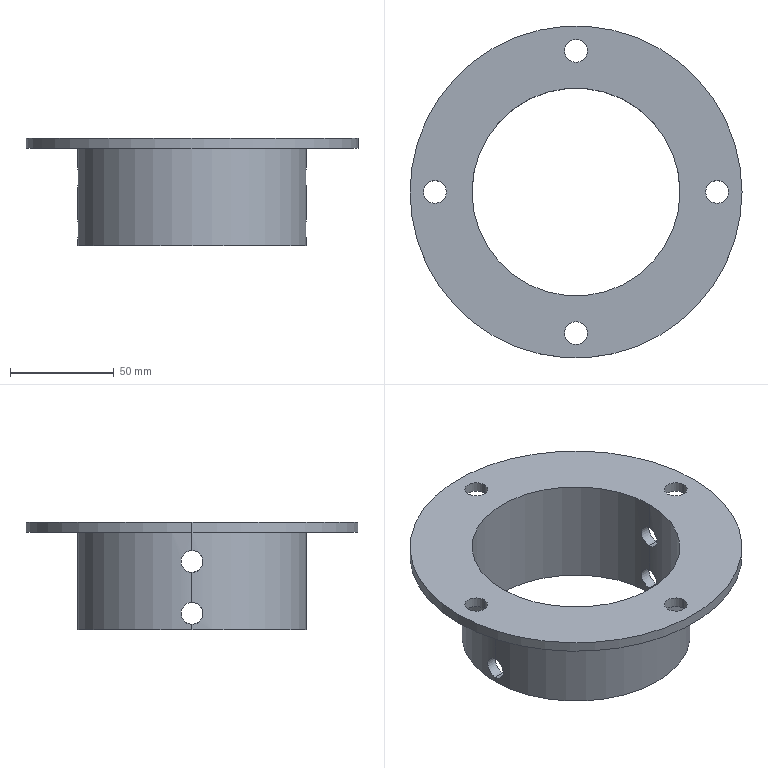Part | SolidWorks | features MirrorStock 1 | 1 solid | 25 faces | box 160 x 160 x 52 mm | volume 135135 mm3 | cylinder 22 | plane 3 | commonest cylinder face diameters 10.5 x8 11 x8 100.2 x2 110.2 x2 160 x2